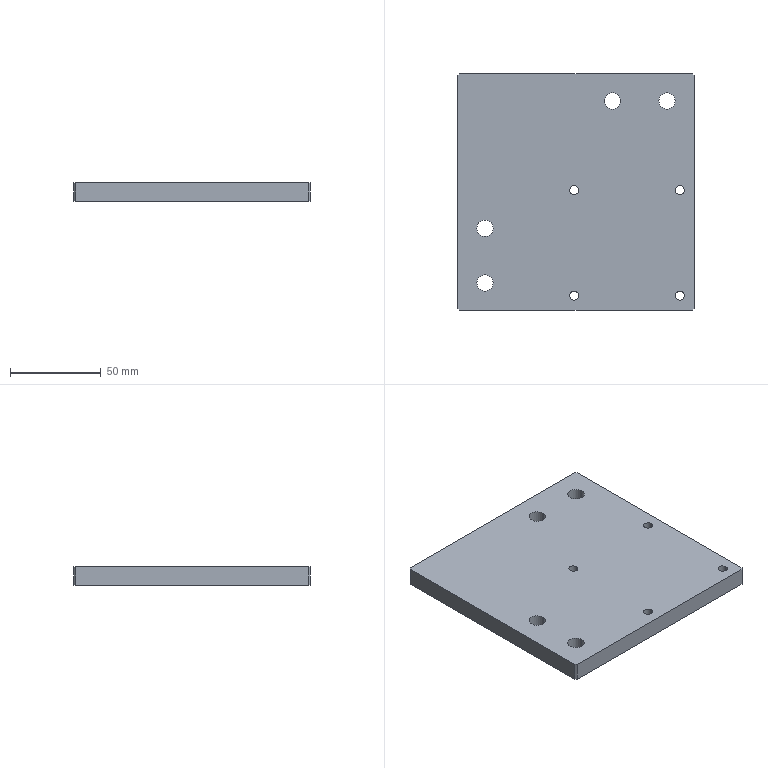Part | STEP file | PN_0010 | 1 solid | 26 faces | box 130 x 130 x 10 mm | volume 165650 mm3 | cylinder 16 | plane 10 | commonest cylinder face diameters 5 x8 9 x8